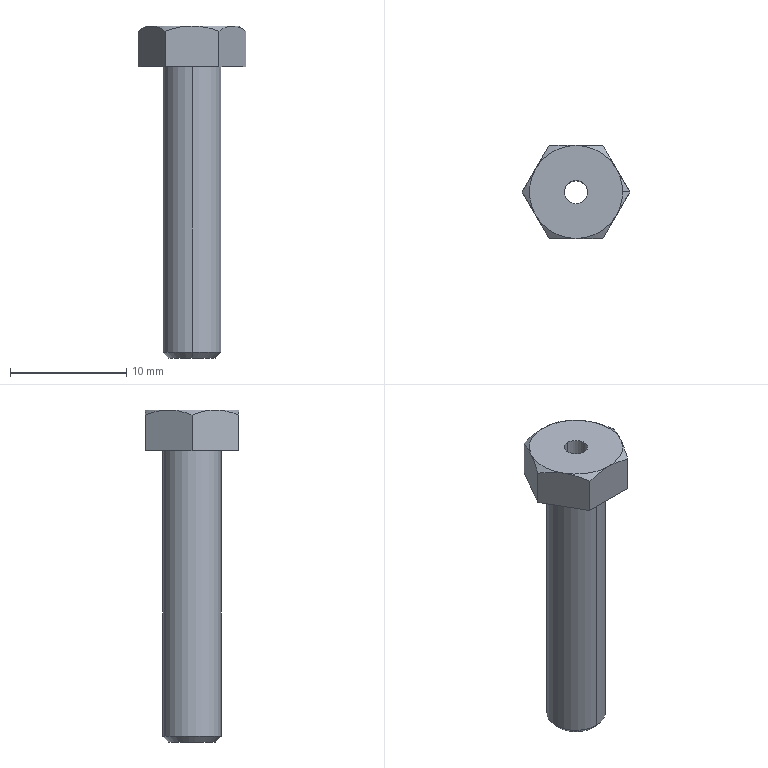Part | SolidWorks | features ICE 2, Chamfer 1, Revolution 1 | 1 solid | 22 faces | box 9.238 x 8 x 28.5 mm | volume 592.822 mm3 | cone 9 | plane 9 | cylinder 4 | commonest cylinder face diameters 2 x2 5 x2
STEP:
#1=CARTESIAN_POINT('',(0.,2.,-25.));
#2=VERTEX_POINT('',#1);
#3=CARTESIAN_POINT('',(0.,-2.,-25.));
#4=VERTEX_POINT('',#3);
#5=CARTESIAN_POINT('',(0.,0.,-25.));
#6=DIRECTION('',(0.,0.,-1.));
#7=DIRECTION('',(0.,-1.,0.));
#8=AXIS2_PLACEMENT_3D('',#5,#6,#7);
#9=CIRCLE('',#8,2.);
#10=EDGE_CURVE('',#2,#4,#9,.T.);
#11=ORIENTED_EDGE('',*,*,#10,.F.);
#12=CARTESIAN_POINT('',(0.,2.5,-24.5));
#13=VERTEX_POINT('',#12);
#14=CARTESIAN_POINT('',(0.,2.5,-24.5));
#15=DIRECTION('',(0.,0.7071,0.7071));
#16=VECTOR('',#15,1000.);
#17=LINE('',#14,#16);
#18=EDGE_CURVE('',#2,#13,#17,.T.);
#19=ORIENTED_EDGE('',*,*,#18,.T.);
#20=CARTESIAN_POINT('',(0.,-2.5,-24.5));
#21=VERTEX_POINT('',#20);
#22=CARTESIAN_POINT('',(0.,0.,-24.5));
#23=DIRECTION('',(0.,0.,1.));
#24=DIRECTION('',(0.,-1.,0.));
#25=AXIS2_PLACEMENT_3D('',#22,#23,#24);
#26=CIRCLE('',#25,2.5);
#27=EDGE_CURVE('',#21,#13,#26,.T.);
#28=ORIENTED_EDGE('',*,*,#27,.F.);
#29=CARTESIAN_POINT('',(0.,-2.5,-24.5));
#30=DIRECTION('',(0.,-0.7071,0.7071));
#31=VECTOR('',#30,1000.);
#32=LINE('',#29,#31);
#33=EDGE_CURVE('',#4,#21,#32,.T.);
#34=ORIENTED_EDGE('',*,*,#33,.F.);
#35=EDGE_LOOP('',(#11,#19,#28,#34));
#36=FACE_OUTER_BOUND('',#35,.T.);
#37=CARTESIAN_POINT('',(0.,0.,-24.5));
#38=DIRECTION('',(0.,0.,1.));
#39=DIRECTION('',(0.,-1.,0.));
#40=AXIS2_PLACEMENT_3D('',#37,#38,#39);
#41=CONICAL_SURFACE('',#40,2.5,0.7854);
#42=ADVANCED_FACE('',(#36),#41,.T.);
#43=CARTESIAN_POINT('',(4.,0.,3.5));
#44=VERTEX_POINT('',#43);
#45=CARTESIAN_POINT('',(3.464,2.,3.5));
#46=VERTEX_POINT('',#45);
#47=CARTESIAN_POINT('',(0.,0.,3.5));
#48=DIRECTION('',(0.,0.,1.));
#49=DIRECTION('',(1.,0.,0.));
#50=AXIS2_PLACEMENT_3D('',#47,#48,#49);
#51=CIRCLE('',#50,4.);
#52=EDGE_CURVE('',#44,#46,#51,.T.);
#53=ORIENTED_EDGE('',*,*,#52,.F.);
#54=CARTESIAN_POINT('',(4.619,0.,3.067));
#55=VERTEX_POINT('',#54);
#56=CARTESIAN_POINT('',(4.,0.,3.5));
#57=DIRECTION('',(0.8192,0.,-0.5736));
#58=VECTOR('',#57,1000.);
#59=LINE('',#56,#58);
#60=EDGE_CURVE('',#44,#55,#59,.T.);
#61=ORIENTED_EDGE('',*,*,#60,.T.);
#62=CARTESIAN_POINT('',(3.464,2.,3.5));
#63=CARTESIAN_POINT('',(3.563,1.829,3.5));
#64=CARTESIAN_POINT('',(3.662,1.657,3.49));
#65=CARTESIAN_POINT('',(3.858,1.318,3.449));
#66=CARTESIAN_POINT('',(3.955,1.15,3.42));
#67=CARTESIAN_POINT('',(4.243,0.6502,3.306));
#68=CARTESIAN_POINT('',(4.432,0.3232,3.197));
#69=CARTESIAN_POINT('',(4.619,0.,3.067));
#70=B_SPLINE_CURVE_WITH_KNOTS('',3,(#62,#63,#64,#65,#66,#67,#68,#69),.UNSPECIFIED.,.F.,.F.,(4,2,2,4),(0.00235,0.002932,0.003515,0.004681),.UNSPECIFIED.);
#71=EDGE_CURVE('',#46,#55,#70,.T.);
#72=ORIENTED_EDGE('',*,*,#71,.F.);
#73=EDGE_LOOP('',(#53,#61,#72));
#74=FACE_OUTER_BOUND('',#73,.T.);
#75=CARTESIAN_POINT('',(0.,0.,3.5));
#76=DIRECTION('',(0.,0.,-1.));
#77=DIRECTION('',(1.,0.,0.));
#78=AXIS2_PLACEMENT_3D('',#75,#76,#77);
#79=CONICAL_SURFACE('',#78,4.,0.9599);
#80=ADVANCED_FACE('',(#74),#79,.T.);
#81=CARTESIAN_POINT('',(0.,1.,-25.));
#82=VERTEX_POINT('',#81);
#83=CARTESIAN_POINT('',(0.,-1.,-25.));
#84=VERTEX_POINT('',#83);
#85=CARTESIAN_POINT('',(0.,0.,-25.));
#86=DIRECTION('',(0.,0.,1.));
#87=DIRECTION('',(0.,-1.,0.));
#88=AXIS2_PLACEMENT_3D('',#85,#86,#87);
#89=CIRCLE('',#88,1.);
#90=EDGE_CURVE('',#82,#84,#89,.T.);
#91=ORIENTED_EDGE('',*,*,#90,.F.);
#92=CARTESIAN_POINT('',(0.,1.,3.5));
#93=VERTEX_POINT('',#92);
#94=CARTESIAN_POINT('',(0.,1.,3.5));
#95=DIRECTION('',(0.,0.,1.));
#96=VECTOR('',#95,1000.);
#97=LINE('',#94,#96);
#98=EDGE_CURVE('',#82,#93,#97,.T.);
#99=ORIENTED_EDGE('',*,*,#98,.T.);
#100=CARTESIAN_POINT('',(0.,-1.,3.5));
#101=VERTEX_POINT('',#100);
#102=CARTESIAN_POINT('',(0.,0.,3.5));
#103=DIRECTION('',(0.,0.,1.));
#104=DIRECTION('',(0.,-1.,0.));
#105=AXIS2_PLACEMENT_3D('',#102,#103,#104);
#106=CIRCLE('',#105,1.);
#107=EDGE_CURVE('',#93,#101,#106,.T.);
#108=ORIENTED_EDGE('',*,*,#107,.T.);
#109=CARTESIAN_POINT('',(0.,-1.,3.5));
#110=DIRECTION('',(0.,0.,1.));
#111=VECTOR('',#110,1000.);
#112=LINE('',#109,#111);
#113=EDGE_CURVE('',#84,#101,#112,.T.);
#114=ORIENTED_EDGE('',*,*,#113,.F.);
#115=EDGE_LOOP('',(#91,#99,#108,#114));
#116=FACE_OUTER_BOUND('',#115,.T.);
#117=CARTESIAN_POINT('',(0.,0.,3.5));
#118=DIRECTION('',(0.,0.,1.));
#119=DIRECTION('',(0.,-1.,0.));
#120=AXIS2_PLACEMENT_3D('',#117,#118,#119);
#121=CYLINDRICAL_SURFACE('',#120,1.);
#122=ADVANCED_FACE('',(#116),#121,.F.);
#123=ORIENTED_EDGE('',*,*,#27,.T.);
#124=CARTESIAN_POINT('',(0.,2.5,0.));
#125=VERTEX_POINT('',#124);
#126=CARTESIAN_POINT('',(0.,2.5,3.5));
#127=DIRECTION('',(0.,0.,1.));
#128=VECTOR('',#127,1000.);
#129=LINE('',#126,#128);
#130=EDGE_CURVE('',#13,#125,#129,.T.);
#131=ORIENTED_EDGE('',*,*,#130,.T.);
#132=CARTESIAN_POINT('',(0.,-2.5,0.));
#133=VERTEX_POINT('',#132);
#134=CARTESIAN_POINT('',(0.,0.,0.));
#135=DIRECTION('',(0.,0.,1.));
#136=DIRECTION('',(1.,0.,0.));
#137=AXIS2_PLACEMENT_3D('',#134,#135,#136);
#138=CIRCLE('',#137,2.5);
#139=EDGE_CURVE('',#133,#125,#138,.T.);
#140=ORIENTED_EDGE('',*,*,#139,.F.);
#141=CARTESIAN_POINT('',(0.,-2.5,3.5));
#142=DIRECTION('',(0.,0.,1.));
#143=VECTOR('',#142,1000.);
#144=LINE('',#141,#143);
#145=EDGE_CURVE('',#21,#133,#144,.T.);
#146=ORIENTED_EDGE('',*,*,#145,.F.);
#147=EDGE_LOOP('',(#123,#131,#140,#146));
#148=FACE_OUTER_BOUND('',#147,.T.);
#149=CARTESIAN_POINT('',(0.,0.,3.5));
#150=DIRECTION('',(0.,0.,1.));
#151=DIRECTION('',(0.,-1.,0.));
#152=AXIS2_PLACEMENT_3D('',#149,#150,#151);
#153=CYLINDRICAL_SURFACE('',#152,2.5);
#154=ADVANCED_FACE('',(#148),#153,.T.);
#155=CARTESIAN_POINT('',(0.,0.,3.5));
#156=DIRECTION('',(0.,0.,1.));
#157=DIRECTION('',(0.,-1.,0.));
#158=AXIS2_PLACEMENT_3D('',#155,#156,#157);
#159=CIRCLE('',#158,1.);
#160=EDGE_CURVE('',#101,#93,#159,.T.);
#161=ORIENTED_EDGE('',*,*,#160,.F.);
#162=ORIENTED_EDGE('',*,*,#107,.F.);
#163=EDGE_LOOP('',(#161,#162));
#164=FACE_BOUND('',#163,.T.);
#165=CARTESIAN_POINT('',(0.,4.,3.5));
#166=VERTEX_POINT('',#165);
#167=CARTESIAN_POINT('',(0.,0.,3.5));
#168=DIRECTION('',(0.,0.,1.));
#169=DIRECTION('',(1.,0.,0.));
#170=AXIS2_PLACEMENT_3D('',#167,#168,#169);
#171=CIRCLE('',#170,4.);
#172=EDGE_CURVE('',#46,#166,#171,.T.);
#173=ORIENTED_EDGE('',*,*,#172,.T.);
#174=CARTESIAN_POINT('',(-3.464,2.,3.5));
#175=VERTEX_POINT('',#174);
#176=CARTESIAN_POINT('',(0.,0.,3.5));
#177=DIRECTION('',(0.,0.,1.));
#178=DIRECTION('',(1.,0.,0.));
#179=AXIS2_PLACEMENT_3D('',#176,#177,#178);
#180=CIRCLE('',#179,4.);
#181=EDGE_CURVE('',#166,#175,#180,.T.);
#182=ORIENTED_EDGE('',*,*,#181,.T.);
#183=CARTESIAN_POINT('',(-3.464,-2.,3.5));
#184=VERTEX_POINT('',#183);
#185=CARTESIAN_POINT('',(0.,0.,3.5));
#186=DIRECTION('',(0.,0.,1.));
#187=DIRECTION('',(1.,0.,0.));
#188=AXIS2_PLACEMENT_3D('',#185,#186,#187);
#189=CIRCLE('',#188,4.);
#190=EDGE_CURVE('',#175,#184,#189,.T.);
#191=ORIENTED_EDGE('',*,*,#190,.T.);
#192=CARTESIAN_POINT('',(0.,-4.,3.5));
#193=VERTEX_POINT('',#192);
#194=CARTESIAN_POINT('',(0.,0.,3.5));
#195=DIRECTION('',(0.,0.,1.));
#196=DIRECTION('',(1.,0.,0.));
#197=AXIS2_PLACEMENT_3D('',#194,#195,#196);
#198=CIRCLE('',#197,4.);
#199=EDGE_CURVE('',#184,#193,#198,.T.);
#200=ORIENTED_EDGE('',*,*,#199,.T.);
#201=CARTESIAN_POINT('',(3.464,-2.,3.5));
#202=VERTEX_POINT('',#201);
#203=CARTESIAN_POINT('',(0.,0.,3.5));
#204=DIRECTION('',(0.,0.,1.));
#205=DIRECTION('',(1.,0.,0.));
#206=AXIS2_PLACEMENT_3D('',#203,#204,#205);
#207=CIRCLE('',#206,4.);
#208=EDGE_CURVE('',#193,#202,#207,.T.);
#209=ORIENTED_EDGE('',*,*,#208,.T.);
#210=CARTESIAN_POINT('',(0.,0.,3.5));
#211=DIRECTION('',(0.,0.,1.));
#212=DIRECTION('',(1.,0.,0.));
#213=AXIS2_PLACEMENT_3D('',#210,#211,#212);
#214=CIRCLE('',#213,4.);
#215=EDGE_CURVE('',#202,#44,#214,.T.);
#216=ORIENTED_EDGE('',*,*,#215,.T.);
#217=ORIENTED_EDGE('',*,*,#52,.T.);
#218=EDGE_LOOP('',(#173,#182,#191,#200,#209,#216,#217));
#219=FACE_OUTER_BOUND('',#218,.T.);
#220=CARTESIAN_POINT('',(0.,2.5,3.5));
#221=DIRECTION('',(0.,0.,-1.));
#222=DIRECTION('',(0.,1.,0.));
#223=AXIS2_PLACEMENT_3D('',#220,#221,#222);
#224=PLANE('',#223);
#225=ADVANCED_FACE('',(#164,#219),#224,.F.);
#226=CARTESIAN_POINT('',(2.309,4.,0.));
#227=VERTEX_POINT('',#226);
#228=CARTESIAN_POINT('',(2.309,4.,3.067));
#229=VERTEX_POINT('',#228);
#230=CARTESIAN_POINT('',(2.309,4.,0.));
#231=DIRECTION('',(0.,0.,1.));
#232=VECTOR('',#231,1000.);
#233=LINE('',#230,#232);
#234=EDGE_CURVE('',#227,#229,#233,.T.);
#235=ORIENTED_EDGE('',*,*,#234,.T.);
#236=CARTESIAN_POINT('',(2.309,4.,3.067));
#237=CARTESIAN_POINT('',(2.684,3.351,3.329));
#238=CARTESIAN_POINT('',(3.067,2.688,3.5));
#239=CARTESIAN_POINT('',(3.464,2.,3.5));
#240=B_SPLINE_CURVE_WITH_KNOTS('',3,(#236,#237,#238,#239),.UNSPECIFIED.,.F.,.F.,(4,4),(0.000000241,0.00235),.UNSPECIFIED.);
#241=EDGE_CURVE('',#229,#46,#240,.T.);
#242=ORIENTED_EDGE('',*,*,#241,.T.);
#243=ORIENTED_EDGE('',*,*,#71,.T.);
#244=CARTESIAN_POINT('',(4.619,0.,0.));
#245=VERTEX_POINT('',#244);
#246=CARTESIAN_POINT('',(4.619,0.,0.));
#247=DIRECTION('',(0.,0.,1.));
#248=VECTOR('',#247,1000.);
#249=LINE('',#246,#248);
#250=EDGE_CURVE('',#245,#55,#249,.T.);
#251=ORIENTED_EDGE('',*,*,#250,.F.);
#252=CARTESIAN_POINT('',(4.619,0.,0.));
#253=DIRECTION('',(-0.5,0.866,0.));
#254=VECTOR('',#253,1000.);
#255=LINE('',#252,#254);
#256=EDGE_CURVE('',#245,#227,#255,.T.);
#257=ORIENTED_EDGE('',*,*,#256,.T.);
#258=EDGE_LOOP('',(#235,#242,#243,#251,#257));
#259=FACE_OUTER_BOUND('',#258,.T.);
#260=CARTESIAN_POINT('',(4.619,0.,0.));
#261=DIRECTION('',(0.866,0.5,0.));
#262=DIRECTION('',(-0.5,0.866,0.));
#263=AXIS2_PLACEMENT_3D('',#260,#261,#262);
#264=PLANE('',#263);
#265=ADVANCED_FACE('',(#259),#264,.T.);
#266=ORIENTED_EDGE('',*,*,#250,.T.);
#267=CARTESIAN_POINT('',(4.619,0.,3.067));
#268=CARTESIAN_POINT('',(4.244,-0.6494,3.329));
#269=CARTESIAN_POINT('',(3.861,-1.312,3.5));
#270=CARTESIAN_POINT('',(3.464,-2.,3.5));
#271=B_SPLINE_CURVE_WITH_KNOTS('',3,(#267,#268,#269,#270),.UNSPECIFIED.,.F.,.F.,(4,4),(0.000000241,0.00235),.UNSPECIFIED.);
#272=EDGE_CURVE('',#55,#202,#271,.T.);
#273=ORIENTED_EDGE('',*,*,#272,.T.);
#274=CARTESIAN_POINT('',(2.309,-4.,3.067));
#275=VERTEX_POINT('',#274);
#276=CARTESIAN_POINT('',(3.464,-2.,3.5));
#277=CARTESIAN_POINT('',(3.366,-2.171,3.5));
#278=CARTESIAN_POINT('',(3.266,-2.343,3.49));
#279=CARTESIAN_POINT('',(3.07,-2.682,3.449));
#280=CARTESIAN_POINT('',(2.973,-2.85,3.42));
#281=CARTESIAN_POINT('',(2.685,-3.35,3.306));
#282=CARTESIAN_POINT('',(2.496,-3.677,3.197));
#283=CARTESIAN_POINT('',(2.309,-4.,3.067));
#284=B_SPLINE_CURVE_WITH_KNOTS('',3,(#276,#277,#278,#279,#280,#281,#282,#283),.UNSPECIFIED.,.F.,.F.,(4,2,2,4),(0.00235,0.002932,0.003515,0.004681),.UNSPECIFIED.);
#285=EDGE_CURVE('',#202,#275,#284,.T.);
#286=ORIENTED_EDGE('',*,*,#285,.T.);
#287=CARTESIAN_POINT('',(2.309,-4.,0.));
#288=VERTEX_POINT('',#287);
#289=CARTESIAN_POINT('',(2.309,-4.,0.));
#290=DIRECTION('',(0.,0.,1.));
#291=VECTOR('',#290,1000.);
#292=LINE('',#289,#291);
#293=EDGE_CURVE('',#288,#275,#292,.T.);
#294=ORIENTED_EDGE('',*,*,#293,.F.);
#295=CARTESIAN_POINT('',(2.309,-4.,0.));
#296=DIRECTION('',(0.5,0.866,0.));
#297=VECTOR('',#296,1000.);
#298=LINE('',#295,#297);
#299=EDGE_CURVE('',#288,#245,#298,.T.);
#300=ORIENTED_EDGE('',*,*,#299,.T.);
#301=EDGE_LOOP('',(#266,#273,#286,#294,#300));
#302=FACE_OUTER_BOUND('',#301,.T.);
#303=CARTESIAN_POINT('',(2.309,-4.,0.));
#304=DIRECTION('',(0.866,-0.5,0.));
#305=DIRECTION('',(0.5,0.866,0.));
#306=AXIS2_PLACEMENT_3D('',#303,#304,#305);
#307=PLANE('',#306);
#308=ADVANCED_FACE('',(#302),#307,.T.);
#309=ORIENTED_EDGE('',*,*,#293,.T.);
#310=CARTESIAN_POINT('',(2.309,-4.,3.067));
#311=CARTESIAN_POINT('',(1.939,-4.,3.196));
#312=CARTESIAN_POINT('',(1.563,-4.,3.305));
#313=CARTESIAN_POINT('',(0.7916,-4.,3.457));
#314=CARTESIAN_POINT('',(0.3924,-4.,3.5));
#315=CARTESIAN_POINT('',(0.,-4.,3.5));
#316=B_SPLINE_CURVE_WITH_KNOTS('',3,(#310,#311,#312,#313,#314,#315),.UNSPECIFIED.,.F.,.F.,(4,2,4),(0.009329,0.01051,0.01168),.UNSPECIFIED.);
#317=EDGE_CURVE('',#275,#193,#316,.T.);
#318=ORIENTED_EDGE('',*,*,#317,.T.);
#319=CARTESIAN_POINT('',(-2.309,-4.,3.067));
#320=VERTEX_POINT('',#319);
#321=CARTESIAN_POINT('',(0.,-4.,3.5));
#322=CARTESIAN_POINT('',(-0.3931,-4.,3.5));
#323=CARTESIAN_POINT('',(-0.7822,-4.,3.459));
#324=CARTESIAN_POINT('',(-1.554,-4.,3.307));
#325=CARTESIAN_POINT('',(-1.938,-4.,3.197));
#326=CARTESIAN_POINT('',(-2.309,-4.,3.067));
#327=B_SPLINE_CURVE_WITH_KNOTS('',3,(#321,#322,#323,#324,#325,#326),.UNSPECIFIED.,.F.,.F.,(4,2,4),(0.01168,0.01286,0.01404),.UNSPECIFIED.);
#328=EDGE_CURVE('',#193,#320,#327,.T.);
#329=ORIENTED_EDGE('',*,*,#328,.T.);
#330=CARTESIAN_POINT('',(-2.309,-4.,0.));
#331=VERTEX_POINT('',#330);
#332=CARTESIAN_POINT('',(-2.309,-4.,0.));
#333=DIRECTION('',(0.,0.,1.));
#334=VECTOR('',#333,1000.);
#335=LINE('',#332,#334);
#336=EDGE_CURVE('',#331,#320,#335,.T.);
#337=ORIENTED_EDGE('',*,*,#336,.F.);
#338=CARTESIAN_POINT('',(-2.309,-4.,0.));
#339=DIRECTION('',(1.,0.,0.));
#340=VECTOR('',#339,1000.);
#341=LINE('',#338,#340);
#342=EDGE_CURVE('',#331,#288,#341,.T.);
#343=ORIENTED_EDGE('',*,*,#342,.T.);
#344=EDGE_LOOP('',(#309,#318,#329,#337,#343));
#345=FACE_OUTER_BOUND('',#344,.T.);
#346=CARTESIAN_POINT('',(-2.309,-4.,0.));
#347=DIRECTION('',(0.,-1.,0.));
#348=DIRECTION('',(0.,0.,-1.));
#349=AXIS2_PLACEMENT_3D('',#346,#347,#348);
#350=PLANE('',#349);
#351=ADVANCED_FACE('',(#345),#350,.T.);
#352=ORIENTED_EDGE('',*,*,#336,.T.);
#353=CARTESIAN_POINT('',(-2.309,-4.,3.067));
#354=CARTESIAN_POINT('',(-2.684,-3.351,3.329));
#355=CARTESIAN_POINT('',(-3.067,-2.688,3.5));
#356=CARTESIAN_POINT('',(-3.464,-2.,3.5));
#357=B_SPLINE_CURVE_WITH_KNOTS('',3,(#353,#354,#355,#356),.UNSPECIFIED.,.F.,.F.,(4,4),(0.000000241,0.00235),.UNSPECIFIED.);
#358=EDGE_CURVE('',#320,#184,#357,.T.);
#359=ORIENTED_EDGE('',*,*,#358,.T.);
#360=CARTESIAN_POINT('',(-4.619,0.,3.067));
#361=VERTEX_POINT('',#360);
#362=CARTESIAN_POINT('',(-3.464,-2.,3.5));
#363=CARTESIAN_POINT('',(-3.563,-1.829,3.5));
#364=CARTESIAN_POINT('',(-3.662,-1.657,3.49));
#365=CARTESIAN_POINT('',(-3.858,-1.318,3.449));
#366=CARTESIAN_POINT('',(-3.955,-1.15,3.42));
#367=CARTESIAN_POINT('',(-4.243,-0.6502,3.306));
#368=CARTESIAN_POINT('',(-4.432,-0.3232,3.197));
#369=CARTESIAN_POINT('',(-4.619,0.,3.067));
#370=B_SPLINE_CURVE_WITH_KNOTS('',3,(#362,#363,#364,#365,#366,#367,#368,#369),.UNSPECIFIED.,.F.,.F.,(4,2,2,4),(0.00235,0.002932,0.003515,0.004681),.UNSPECIFIED.);
#371=EDGE_CURVE('',#184,#361,#370,.T.);
#372=ORIENTED_EDGE('',*,*,#371,.T.);
#373=CARTESIAN_POINT('',(-4.619,0.,0.));
#374=VERTEX_POINT('',#373);
#375=CARTESIAN_POINT('',(-4.619,0.,0.));
#376=DIRECTION('',(0.,0.,1.));
#377=VECTOR('',#376,1000.);
#378=LINE('',#375,#377);
#379=EDGE_CURVE('',#374,#361,#378,.T.);
#380=ORIENTED_EDGE('',*,*,#379,.F.);
#381=CARTESIAN_POINT('',(-4.619,0.,0.));
#382=DIRECTION('',(0.5,-0.866,0.));
#383=VECTOR('',#382,1000.);
#384=LINE('',#381,#383);
#385=EDGE_CURVE('',#374,#331,#384,.T.);
#386=ORIENTED_EDGE('',*,*,#385,.T.);
#387=EDGE_LOOP('',(#352,#359,#372,#380,#386));
#388=FACE_OUTER_BOUND('',#387,.T.);
#389=CARTESIAN_POINT('',(-4.619,0.,0.));
#390=DIRECTION('',(-0.866,-0.5,0.));
#391=DIRECTION('',(0.5,-0.866,0.));
#392=AXIS2_PLACEMENT_3D('',#389,#390,#391);
#393=PLANE('',#392);
#394=ADVANCED_FACE('',(#388),#393,.T.);
#395=ORIENTED_EDGE('',*,*,#379,.T.);
#396=CARTESIAN_POINT('',(-4.619,0.,3.067));
#397=CARTESIAN_POINT('',(-4.244,0.6494,3.329));
#398=CARTESIAN_POINT('',(-3.861,1.312,3.5));
#399=CARTESIAN_POINT('',(-3.464,2.,3.5));
#400=B_SPLINE_CURVE_WITH_KNOTS('',3,(#396,#397,#398,#399),.UNSPECIFIED.,.F.,.F.,(4,4),(0.000000241,0.00235),.UNSPECIFIED.);
#401=EDGE_CURVE('',#361,#175,#400,.T.);
#402=ORIENTED_EDGE('',*,*,#401,.T.);
#403=CARTESIAN_POINT('',(-2.309,4.,3.067));
#404=VERTEX_POINT('',#403);
#405=CARTESIAN_POINT('',(-3.464,2.,3.5));
#406=CARTESIAN_POINT('',(-3.366,2.171,3.5));
#407=CARTESIAN_POINT('',(-3.266,2.343,3.49));
#408=CARTESIAN_POINT('',(-3.07,2.682,3.449));
#409=CARTESIAN_POINT('',(-2.973,2.85,3.42));
#410=CARTESIAN_POINT('',(-2.685,3.35,3.306));
#411=CARTESIAN_POINT('',(-2.496,3.677,3.197));
#412=CARTESIAN_POINT('',(-2.309,4.,3.067));
#413=B_SPLINE_CURVE_WITH_KNOTS('',3,(#405,#406,#407,#408,#409,#410,#411,#412),.UNSPECIFIED.,.F.,.F.,(4,2,2,4),(0.00235,0.002932,0.003515,0.004681),.UNSPECIFIED.);
#414=EDGE_CURVE('',#175,#404,#413,.T.);
#415=ORIENTED_EDGE('',*,*,#414,.T.);
#416=CARTESIAN_POINT('',(-2.309,4.,0.));
#417=VERTEX_POINT('',#416);
#418=CARTESIAN_POINT('',(-2.309,4.,0.));
#419=DIRECTION('',(0.,0.,1.));
#420=VECTOR('',#419,1000.);
#421=LINE('',#418,#420);
#422=EDGE_CURVE('',#417,#404,#421,.T.);
#423=ORIENTED_EDGE('',*,*,#422,.F.);
#424=CARTESIAN_POINT('',(-2.309,4.,0.));
#425=DIRECTION('',(-0.5,-0.866,0.));
#426=VECTOR('',#425,1000.);
#427=LINE('',#424,#426);
#428=EDGE_CURVE('',#417,#374,#427,.T.);
#429=ORIENTED_EDGE('',*,*,#428,.T.);
#430=EDGE_LOOP('',(#395,#402,#415,#423,#429));
#431=FACE_OUTER_BOUND('',#430,.T.);
#432=CARTESIAN_POINT('',(-2.309,4.,0.));
#433=DIRECTION('',(-0.866,0.5,0.));
#434=DIRECTION('',(-0.5,-0.866,0.));
#435=AXIS2_PLACEMENT_3D('',#432,#433,#434);
#436=PLANE('',#435);
#437=ADVANCED_FACE('',(#431),#436,.T.);
#438=ORIENTED_EDGE('',*,*,#422,.T.);
#439=CARTESIAN_POINT('',(-2.309,4.,3.067));
#440=CARTESIAN_POINT('',(-1.938,4.,3.197));
#441=CARTESIAN_POINT('',(-1.554,4.,3.307));
#442=CARTESIAN_POINT('',(-0.7822,4.,3.459));
#443=CARTESIAN_POINT('',(-0.3931,4.,3.5));
#444=CARTESIAN_POINT('',(0.,4.,3.5));
#445=B_SPLINE_CURVE_WITH_KNOTS('',3,(#439,#440,#441,#442,#443,#444),.UNSPECIFIED.,.F.,.F.,(4,2,4),(0.003696,0.004872,0.006049),.UNSPECIFIED.);
#446=EDGE_CURVE('',#404,#166,#445,.T.);
#447=ORIENTED_EDGE('',*,*,#446,.T.);
#448=CARTESIAN_POINT('',(0.,4.,3.5));
#449=CARTESIAN_POINT('',(0.3924,4.,3.5));
#450=CARTESIAN_POINT('',(0.7916,4.,3.457));
#451=CARTESIAN_POINT('',(1.563,4.,3.305));
#452=CARTESIAN_POINT('',(1.939,4.,3.196));
#453=CARTESIAN_POINT('',(2.309,4.,3.067));
#454=B_SPLINE_CURVE_WITH_KNOTS('',3,(#448,#449,#450,#451,#452,#453),.UNSPECIFIED.,.F.,.F.,(4,2,4),(0.006049,0.007223,0.008398),.UNSPECIFIED.);
#455=EDGE_CURVE('',#166,#229,#454,.T.);
#456=ORIENTED_EDGE('',*,*,#455,.T.);
#457=ORIENTED_EDGE('',*,*,#234,.F.);
#458=CARTESIAN_POINT('',(2.309,4.,0.));
#459=DIRECTION('',(-1.,0.,0.));
#460=VECTOR('',#459,1000.);
#461=LINE('',#458,#460);
#462=EDGE_CURVE('',#227,#417,#461,.T.);
#463=ORIENTED_EDGE('',*,*,#462,.T.);
#464=EDGE_LOOP('',(#438,#447,#456,#457,#463));
#465=FACE_OUTER_BOUND('',#464,.T.);
#466=CARTESIAN_POINT('',(2.309,4.,0.));
#467=DIRECTION('',(0.,1.,0.));
#468=DIRECTION('',(0.,0.,1.));
#469=AXIS2_PLACEMENT_3D('',#466,#467,#468);
#470=PLANE('',#469);
#471=ADVANCED_FACE('',(#465),#470,.T.);
#472=ORIENTED_EDGE('',*,*,#130,.F.);
#473=CARTESIAN_POINT('',(0.,0.,-24.5));
#474=DIRECTION('',(0.,0.,1.));
#475=DIRECTION('',(0.,-1.,0.));
#476=AXIS2_PLACEMENT_3D('',#473,#474,#475);
#477=CIRCLE('',#476,2.5);
#478=EDGE_CURVE('',#13,#21,#477,.T.);
#479=ORIENTED_EDGE('',*,*,#478,.T.);
#480=ORIENTED_EDGE('',*,*,#145,.T.);
#481=CARTESIAN_POINT('',(0.,0.,0.));
#482=DIRECTION('',(0.,0.,1.));
#483=DIRECTION('',(1.,0.,0.));
#484=AXIS2_PLACEMENT_3D('',#481,#482,#483);
#485=CIRCLE('',#484,2.5);
#486=EDGE_CURVE('',#125,#133,#485,.T.);
#487=ORIENTED_EDGE('',*,*,#486,.F.);
#488=EDGE_LOOP('',(#472,#479,#480,#487));
#489=FACE_OUTER_BOUND('',#488,.T.);
#490=CARTESIAN_POINT('',(0.,0.,3.5));
#491=DIRECTION('',(0.,0.,1.));
#492=DIRECTION('',(0.,-1.,0.));
#493=AXIS2_PLACEMENT_3D('',#490,#491,#492);
#494=CYLINDRICAL_SURFACE('',#493,2.5);
#495=ADVANCED_FACE('',(#489),#494,.T.);
#496=CARTESIAN_POINT('',(0.,0.,-25.));
#497=DIRECTION('',(0.,0.,-1.));
#498=DIRECTION('',(0.,-1.,0.));
#499=AXIS2_PLACEMENT_3D('',#496,#497,#498);
#500=CIRCLE('',#499,2.);
#501=EDGE_CURVE('',#4,#2,#500,.T.);
#502=ORIENTED_EDGE('',*,*,#501,.T.);
#503=ORIENTED_EDGE('',*,*,#10,.T.);
#504=EDGE_LOOP('',(#502,#503));
#505=FACE_OUTER_BOUND('',#504,.T.);
#506=CARTESIAN_POINT('',(0.,0.,-25.));
#507=DIRECTION('',(0.,0.,1.));
#508=DIRECTION('',(0.,-1.,0.));
#509=AXIS2_PLACEMENT_3D('',#506,#507,#508);
#510=CIRCLE('',#509,1.);
#511=EDGE_CURVE('',#84,#82,#510,.T.);
#512=ORIENTED_EDGE('',*,*,#511,.T.);
#513=ORIENTED_EDGE('',*,*,#90,.T.);
#514=EDGE_LOOP('',(#512,#513));
#515=FACE_BOUND('',#514,.T.);
#516=CARTESIAN_POINT('',(0.,2.5,-25.));
#517=DIRECTION('',(0.,0.,1.));
#518=DIRECTION('',(0.,-1.,0.));
#519=AXIS2_PLACEMENT_3D('',#516,#517,#518);
#520=PLANE('',#519);
#521=ADVANCED_FACE('',(#505,#515),#520,.F.);
#522=ORIENTED_EDGE('',*,*,#98,.F.);
#523=ORIENTED_EDGE('',*,*,#511,.F.);
#524=ORIENTED_EDGE('',*,*,#113,.T.);
#525=ORIENTED_EDGE('',*,*,#160,.T.);
#526=EDGE_LOOP('',(#522,#523,#524,#525));
#527=FACE_OUTER_BOUND('',#526,.T.);
#528=CARTESIAN_POINT('',(0.,0.,3.5));
#529=DIRECTION('',(0.,0.,1.));
#530=DIRECTION('',(0.,-1.,0.));
#531=AXIS2_PLACEMENT_3D('',#528,#529,#530);
#532=CYLINDRICAL_SURFACE('',#531,1.);
#533=ADVANCED_FACE('',(#527),#532,.F.);
#534=ORIENTED_EDGE('',*,*,#256,.F.);
#535=ORIENTED_EDGE('',*,*,#299,.F.);
#536=ORIENTED_EDGE('',*,*,#342,.F.);
#537=ORIENTED_EDGE('',*,*,#385,.F.);
#538=ORIENTED_EDGE('',*,*,#428,.F.);
#539=ORIENTED_EDGE('',*,*,#462,.F.);
#540=EDGE_LOOP('',(#534,#535,#536,#537,#538,#539));
#541=FACE_OUTER_BOUND('',#540,.T.);
#542=ORIENTED_EDGE('',*,*,#139,.T.);
#543=ORIENTED_EDGE('',*,*,#486,.T.);
#544=EDGE_LOOP('',(#542,#543));
#545=FACE_BOUND('',#544,.T.);
#546=CARTESIAN_POINT('',(2.309,4.,0.));
#547=DIRECTION('',(0.,0.,1.));
#548=DIRECTION('',(1.,0.,0.));
#549=AXIS2_PLACEMENT_3D('',#546,#547,#548);
#550=PLANE('',#549);
#551=ADVANCED_FACE('',(#541,#545),#550,.F.);
#552=ORIENTED_EDGE('',*,*,#455,.F.);
#553=ORIENTED_EDGE('',*,*,#172,.F.);
#554=ORIENTED_EDGE('',*,*,#241,.F.);
#555=EDGE_LOOP('',(#552,#553,#554));
#556=FACE_OUTER_BOUND('',#555,.T.);
#557=CARTESIAN_POINT('',(0.,0.,3.5));
#558=DIRECTION('',(0.,0.,-1.));
#559=DIRECTION('',(1.,0.,0.));
#560=AXIS2_PLACEMENT_3D('',#557,#558,#559);
#561=CONICAL_SURFACE('',#560,4.,0.9599);
#562=ADVANCED_FACE('',(#556),#561,.T.);
#563=ORIENTED_EDGE('',*,*,#181,.F.);
#564=ORIENTED_EDGE('',*,*,#446,.F.);
#565=ORIENTED_EDGE('',*,*,#414,.F.);
#566=EDGE_LOOP('',(#563,#564,#565));
#567=FACE_OUTER_BOUND('',#566,.T.);
#568=CARTESIAN_POINT('',(0.,0.,3.5));
#569=DIRECTION('',(0.,0.,-1.));
#570=DIRECTION('',(1.,0.,0.));
#571=AXIS2_PLACEMENT_3D('',#568,#569,#570);
#572=CONICAL_SURFACE('',#571,4.,0.9599);
#573=ADVANCED_FACE('',(#567),#572,.T.);
#574=ORIENTED_EDGE('',*,*,#190,.F.);
#575=ORIENTED_EDGE('',*,*,#401,.F.);
#576=ORIENTED_EDGE('',*,*,#371,.F.);
#577=EDGE_LOOP('',(#574,#575,#576));
#578=FACE_OUTER_BOUND('',#577,.T.);
#579=CARTESIAN_POINT('',(0.,0.,3.5));
#580=DIRECTION('',(0.,0.,-1.));
#581=DIRECTION('',(1.,0.,0.));
#582=AXIS2_PLACEMENT_3D('',#579,#580,#581);
#583=CONICAL_SURFACE('',#582,4.,0.9599);
#584=ADVANCED_FACE('',(#578),#583,.T.);
#585=ORIENTED_EDGE('',*,*,#199,.F.);
#586=ORIENTED_EDGE('',*,*,#358,.F.);
#587=ORIENTED_EDGE('',*,*,#328,.F.);
#588=EDGE_LOOP('',(#585,#586,#587));
#589=FACE_OUTER_BOUND('',#588,.T.);
#590=CARTESIAN_POINT('',(0.,0.,3.5));
#591=DIRECTION('',(0.,0.,-1.));
#592=DIRECTION('',(1.,0.,0.));
#593=AXIS2_PLACEMENT_3D('',#590,#591,#592);
#594=CONICAL_SURFACE('',#593,4.,0.9599);
#595=ADVANCED_FACE('',(#589),#594,.T.);
#596=ORIENTED_EDGE('',*,*,#208,.F.);
#597=ORIENTED_EDGE('',*,*,#317,.F.);
#598=ORIENTED_EDGE('',*,*,#285,.F.);
#599=EDGE_LOOP('',(#596,#597,#598));
#600=FACE_OUTER_BOUND('',#599,.T.);
#601=CARTESIAN_POINT('',(0.,0.,3.5));
#602=DIRECTION('',(0.,0.,-1.));
#603=DIRECTION('',(1.,0.,0.));
#604=AXIS2_PLACEMENT_3D('',#601,#602,#603);
#605=CONICAL_SURFACE('',#604,4.,0.9599);
#606=ADVANCED_FACE('',(#600),#605,.T.);
#607=ORIENTED_EDGE('',*,*,#60,.F.);
#608=ORIENTED_EDGE('',*,*,#215,.F.);
#609=ORIENTED_EDGE('',*,*,#272,.F.);
#610=EDGE_LOOP('',(#607,#608,#609));
#611=FACE_OUTER_BOUND('',#610,.T.);
#612=CARTESIAN_POINT('',(0.,0.,3.5));
#613=DIRECTION('',(0.,0.,-1.));
#614=DIRECTION('',(1.,0.,0.));
#615=AXIS2_PLACEMENT_3D('',#612,#613,#614);
#616=CONICAL_SURFACE('',#615,4.,0.9599);
#617=ADVANCED_FACE('',(#611),#616,.T.);
#618=ORIENTED_EDGE('',*,*,#18,.F.);
#619=ORIENTED_EDGE('',*,*,#501,.F.);
#620=ORIENTED_EDGE('',*,*,#33,.T.);
#621=ORIENTED_EDGE('',*,*,#478,.F.);
#622=EDGE_LOOP('',(#618,#619,#620,#621));
#623=FACE_OUTER_BOUND('',#622,.T.);
#624=CARTESIAN_POINT('',(0.,0.,-24.5));
#625=DIRECTION('',(0.,0.,1.));
#626=DIRECTION('',(0.,-1.,0.));
#627=AXIS2_PLACEMENT_3D('',#624,#625,#626);
#628=CONICAL_SURFACE('',#627,2.5,0.7854);
#629=ADVANCED_FACE('',(#623),#628,.T.);
#630=CLOSED_SHELL('',(#42,#80,#122,#154,#225,#265,#308,#351,#394,#437,#471,#495,#521,#533,#551,#562,#573,#584,#595,#606,#617,#629));
#631=MANIFOLD_SOLID_BREP('',#630);
#632=CARTESIAN_POINT('',(0.,0.,0.));
#633=DIRECTION('',(0.,0.,1.));
#634=DIRECTION('',(1.,0.,0.));
#635=AXIS2_PLACEMENT_3D('',#632,#633,#634);
#636=(LENGTH_UNIT()NAMED_UNIT(*)SI_UNIT(.MILLI.,.METRE.));
#637=UNCERTAINTY_MEASURE_WITH_UNIT(LENGTH_MEASURE(0.00001),#636,'','');
#638=(NAMED_UNIT(*)PLANE_ANGLE_UNIT()SI_UNIT($,.RADIAN.));
#639=(NAMED_UNIT(*)SI_UNIT($,.STERADIAN.)SOLID_ANGLE_UNIT());
#640=(GEOMETRIC_REPRESENTATION_CONTEXT(3)GLOBAL_UNCERTAINTY_ASSIGNED_CONTEXT((#637))GLOBAL_UNIT_ASSIGNED_CONTEXT((#636,#638,#639))REPRESENTATION_CONTEXT('',''));
#641=ADVANCED_BREP_SHAPE_REPRESENTATION('',(#631,#635),#640);